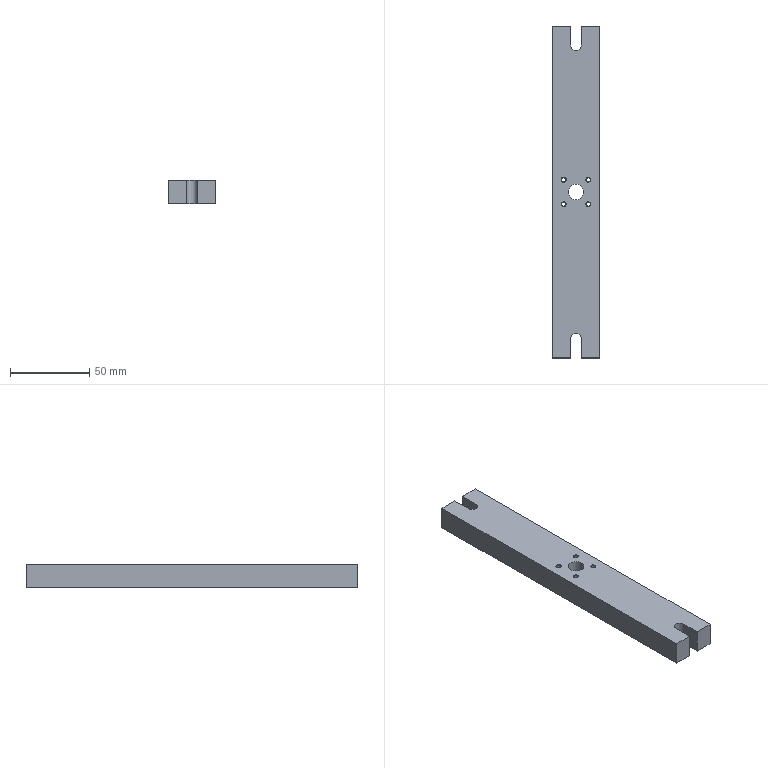Part | STEP file | 200 mesh_id1942 | 1 solid | 32 faces | box 30 x 210 x 15 mm | volume 89577 mm3 | plane 16 | cylinder 11 | cone 5 | commonest cylinder face diameters 2.5 x4 4.5 x4 7 x2 10 x1
STEP:
#1=CARTESIAN_POINT('',(-16645.224,-4012.519,101.75));
#2=VERTEX_POINT('',#1);
#3=CARTESIAN_POINT('',(-16643.974,-4012.519,101.75));
#4=DIRECTION('',(0.,0.,1.));
#5=DIRECTION('',(-1.,0.,0.));
#6=AXIS2_PLACEMENT_3D('',#3,#4,#5);
#7=CIRCLE('',#6,1.25);
#8=EDGE_CURVE('',#2,#2,#7,.T.);
#9=ORIENTED_EDGE('',*,*,#8,.T.);
#10=EDGE_LOOP('',(#9));
#11=FACE_BOUND('',#10,.T.);
#12=CARTESIAN_POINT('',(-16645.224,-4012.519,95.));
#13=VERTEX_POINT('',#12);
#14=CARTESIAN_POINT('',(-16643.974,-4012.519,95.));
#15=DIRECTION('',(0.,0.,1.));
#16=DIRECTION('',(-1.,0.,0.));
#17=AXIS2_PLACEMENT_3D('',#14,#15,#16);
#18=CIRCLE('',#17,1.25);
#19=EDGE_CURVE('',#13,#13,#18,.T.);
#20=ORIENTED_EDGE('',*,*,#19,.F.);
#21=EDGE_LOOP('',(#20));
#22=FACE_BOUND('',#21,.T.);
#23=CARTESIAN_POINT('',(-16643.974,-4012.519,102.));
#24=DIRECTION('',(0.,0.,-1.));
#25=DIRECTION('',(-1.,0.,0.));
#26=AXIS2_PLACEMENT_3D('',#23,#24,#25);
#27=CYLINDRICAL_SURFACE('',#26,1.25);
#28=ADVANCED_FACE('',(#11,#22),#27,.F.);
#29=CARTESIAN_POINT('',(-16629.724,-4012.519,101.75));
#30=VERTEX_POINT('',#29);
#31=CARTESIAN_POINT('',(-16628.474,-4012.519,101.75));
#32=DIRECTION('',(0.,0.,1.));
#33=DIRECTION('',(-1.,0.,0.));
#34=AXIS2_PLACEMENT_3D('',#31,#32,#33);
#35=CIRCLE('',#34,1.25);
#36=EDGE_CURVE('',#30,#30,#35,.T.);
#37=ORIENTED_EDGE('',*,*,#36,.T.);
#38=EDGE_LOOP('',(#37));
#39=FACE_BOUND('',#38,.T.);
#40=CARTESIAN_POINT('',(-16629.724,-4012.519,95.));
#41=VERTEX_POINT('',#40);
#42=CARTESIAN_POINT('',(-16628.474,-4012.519,95.));
#43=DIRECTION('',(0.,0.,1.));
#44=DIRECTION('',(-1.,0.,0.));
#45=AXIS2_PLACEMENT_3D('',#42,#43,#44);
#46=CIRCLE('',#45,1.25);
#47=EDGE_CURVE('',#41,#41,#46,.T.);
#48=ORIENTED_EDGE('',*,*,#47,.F.);
#49=EDGE_LOOP('',(#48));
#50=FACE_BOUND('',#49,.T.);
#51=CARTESIAN_POINT('',(-16628.474,-4012.519,102.));
#52=DIRECTION('',(0.,0.,-1.));
#53=DIRECTION('',(-1.,0.,0.));
#54=AXIS2_PLACEMENT_3D('',#51,#52,#53);
#55=CYLINDRICAL_SURFACE('',#54,1.25);
#56=ADVANCED_FACE('',(#39,#50),#55,.F.);
#57=CARTESIAN_POINT('',(-16645.224,-4028.019,101.75));
#58=VERTEX_POINT('',#57);
#59=CARTESIAN_POINT('',(-16643.974,-4028.019,101.75));
#60=DIRECTION('',(0.,0.,1.));
#61=DIRECTION('',(-1.,0.,0.));
#62=AXIS2_PLACEMENT_3D('',#59,#60,#61);
#63=CIRCLE('',#62,1.25);
#64=EDGE_CURVE('',#58,#58,#63,.T.);
#65=ORIENTED_EDGE('',*,*,#64,.T.);
#66=EDGE_LOOP('',(#65));
#67=FACE_BOUND('',#66,.T.);
#68=CARTESIAN_POINT('',(-16645.224,-4028.019,95.));
#69=VERTEX_POINT('',#68);
#70=CARTESIAN_POINT('',(-16643.974,-4028.019,95.));
#71=DIRECTION('',(0.,0.,1.));
#72=DIRECTION('',(-1.,0.,0.));
#73=AXIS2_PLACEMENT_3D('',#70,#71,#72);
#74=CIRCLE('',#73,1.25);
#75=EDGE_CURVE('',#69,#69,#74,.T.);
#76=ORIENTED_EDGE('',*,*,#75,.F.);
#77=EDGE_LOOP('',(#76));
#78=FACE_BOUND('',#77,.T.);
#79=CARTESIAN_POINT('',(-16643.974,-4028.019,102.));
#80=DIRECTION('',(0.,0.,-1.));
#81=DIRECTION('',(-1.,0.,0.));
#82=AXIS2_PLACEMENT_3D('',#79,#80,#81);
#83=CYLINDRICAL_SURFACE('',#82,1.25);
#84=ADVANCED_FACE('',(#67,#78),#83,.F.);
#85=CARTESIAN_POINT('',(-16629.724,-4028.019,101.75));
#86=VERTEX_POINT('',#85);
#87=CARTESIAN_POINT('',(-16628.474,-4028.019,101.75));
#88=DIRECTION('',(0.,0.,1.));
#89=DIRECTION('',(-1.,0.,0.));
#90=AXIS2_PLACEMENT_3D('',#87,#88,#89);
#91=CIRCLE('',#90,1.25);
#92=EDGE_CURVE('',#86,#86,#91,.T.);
#93=ORIENTED_EDGE('',*,*,#92,.T.);
#94=EDGE_LOOP('',(#93));
#95=FACE_BOUND('',#94,.T.);
#96=CARTESIAN_POINT('',(-16629.724,-4028.019,95.));
#97=VERTEX_POINT('',#96);
#98=CARTESIAN_POINT('',(-16628.474,-4028.019,95.));
#99=DIRECTION('',(0.,0.,1.));
#100=DIRECTION('',(-1.,0.,0.));
#101=AXIS2_PLACEMENT_3D('',#98,#99,#100);
#102=CIRCLE('',#101,1.25);
#103=EDGE_CURVE('',#97,#97,#102,.T.);
#104=ORIENTED_EDGE('',*,*,#103,.F.);
#105=EDGE_LOOP('',(#104));
#106=FACE_BOUND('',#105,.T.);
#107=CARTESIAN_POINT('',(-16628.474,-4028.019,102.));
#108=DIRECTION('',(0.,0.,-1.));
#109=DIRECTION('',(-1.,0.,0.));
#110=AXIS2_PLACEMENT_3D('',#107,#108,#109);
#111=CYLINDRICAL_SURFACE('',#110,1.25);
#112=ADVANCED_FACE('',(#95,#106),#111,.F.);
#113=CARTESIAN_POINT('',(-16639.724,-3927.269,102.));
#114=VERTEX_POINT('',#113);
#115=CARTESIAN_POINT('',(-16639.724,-3927.269,87.));
#116=VERTEX_POINT('',#115);
#117=CARTESIAN_POINT('',(-16639.724,-3927.269,146.));
#118=DIRECTION('',(0.,0.,-1.));
#119=VECTOR('',#118,1.);
#120=LINE('',#117,#119);
#121=EDGE_CURVE('',#114,#116,#120,.T.);
#122=ORIENTED_EDGE('',*,*,#121,.T.);
#123=CARTESIAN_POINT('',(-16639.724,-3915.269,87.));
#124=VERTEX_POINT('',#123);
#125=CARTESIAN_POINT('',(-16639.724,-3907.666,87.));
#126=DIRECTION('',(0.,-1.,0.));
#127=VECTOR('',#126,1.);
#128=LINE('',#125,#127);
#129=EDGE_CURVE('',#124,#116,#128,.T.);
#130=ORIENTED_EDGE('',*,*,#129,.F.);
#131=CARTESIAN_POINT('',(-16639.724,-3915.269,102.));
#132=VERTEX_POINT('',#131);
#133=CARTESIAN_POINT('',(-16639.724,-3915.269,146.));
#134=DIRECTION('',(0.,0.,-1.));
#135=VECTOR('',#134,1.);
#136=LINE('',#133,#135);
#137=EDGE_CURVE('',#132,#124,#136,.T.);
#138=ORIENTED_EDGE('',*,*,#137,.F.);
#139=CARTESIAN_POINT('',(-16639.724,-3907.666,102.));
#140=DIRECTION('',(0.,1.,0.));
#141=VECTOR('',#140,1.);
#142=LINE('',#139,#141);
#143=EDGE_CURVE('',#114,#132,#142,.T.);
#144=ORIENTED_EDGE('',*,*,#143,.F.);
#145=EDGE_LOOP('',(#122,#130,#138,#144));
#146=FACE_OUTER_BOUND('',#145,.T.);
#147=CARTESIAN_POINT('',(-16639.724,-3907.666,146.));
#148=DIRECTION('',(-1.,0.,0.));
#149=DIRECTION('',(0.,0.,1.));
#150=AXIS2_PLACEMENT_3D('',#147,#148,#149);
#151=PLANE('',#150);
#152=ADVANCED_FACE('',(#146),#151,.F.);
#153=CARTESIAN_POINT('',(-16632.724,-3915.269,87.));
#154=VERTEX_POINT('',#153);
#155=CARTESIAN_POINT('',(-16632.724,-3915.269,102.));
#156=VERTEX_POINT('',#155);
#157=CARTESIAN_POINT('',(-16632.724,-3915.269,146.));
#158=DIRECTION('',(0.,0.,1.));
#159=VECTOR('',#158,1.);
#160=LINE('',#157,#159);
#161=EDGE_CURVE('',#154,#156,#160,.T.);
#162=ORIENTED_EDGE('',*,*,#161,.F.);
#163=CARTESIAN_POINT('',(-16632.724,-3927.269,87.));
#164=VERTEX_POINT('',#163);
#165=CARTESIAN_POINT('',(-16632.724,-3927.269,87.));
#166=DIRECTION('',(0.,1.,0.));
#167=VECTOR('',#166,1.);
#168=LINE('',#165,#167);
#169=EDGE_CURVE('',#164,#154,#168,.T.);
#170=ORIENTED_EDGE('',*,*,#169,.F.);
#171=CARTESIAN_POINT('',(-16632.724,-3927.269,102.));
#172=VERTEX_POINT('',#171);
#173=CARTESIAN_POINT('',(-16632.724,-3927.269,146.));
#174=DIRECTION('',(0.,0.,-1.));
#175=VECTOR('',#174,1.);
#176=LINE('',#173,#175);
#177=EDGE_CURVE('',#172,#164,#176,.T.);
#178=ORIENTED_EDGE('',*,*,#177,.F.);
#179=CARTESIAN_POINT('',(-16632.724,-3927.269,102.));
#180=DIRECTION('',(0.,-1.,0.));
#181=VECTOR('',#180,1.);
#182=LINE('',#179,#181);
#183=EDGE_CURVE('',#156,#172,#182,.T.);
#184=ORIENTED_EDGE('',*,*,#183,.F.);
#185=EDGE_LOOP('',(#162,#170,#178,#184));
#186=FACE_OUTER_BOUND('',#185,.T.);
#187=CARTESIAN_POINT('',(-16632.724,-3927.269,146.));
#188=DIRECTION('',(1.,0.,0.));
#189=DIRECTION('',(0.,0.,-1.));
#190=AXIS2_PLACEMENT_3D('',#187,#188,#189);
#191=PLANE('',#190);
#192=ADVANCED_FACE('',(#186),#191,.F.);
#193=ORIENTED_EDGE('',*,*,#177,.T.);
#194=CARTESIAN_POINT('',(-16636.224,-3927.269,87.));
#195=DIRECTION('',(0.,0.,-1.));
#196=DIRECTION('',(-1.,0.,0.));
#197=AXIS2_PLACEMENT_3D('',#194,#195,#196);
#198=CIRCLE('',#197,3.5);
#199=EDGE_CURVE('',#164,#116,#198,.T.);
#200=ORIENTED_EDGE('',*,*,#199,.T.);
#201=ORIENTED_EDGE('',*,*,#121,.F.);
#202=CARTESIAN_POINT('',(-16636.224,-3927.269,102.));
#203=DIRECTION('',(0.,0.,-1.));
#204=DIRECTION('',(-1.,0.,0.));
#205=AXIS2_PLACEMENT_3D('',#202,#203,#204);
#206=CIRCLE('',#205,3.5);
#207=EDGE_CURVE('',#172,#114,#206,.T.);
#208=ORIENTED_EDGE('',*,*,#207,.F.);
#209=EDGE_LOOP('',(#193,#200,#201,#208));
#210=FACE_OUTER_BOUND('',#209,.T.);
#211=CARTESIAN_POINT('',(-16636.224,-3927.269,146.));
#212=DIRECTION('',(0.,0.,-1.));
#213=DIRECTION('',(-1.,0.,0.));
#214=AXIS2_PLACEMENT_3D('',#211,#212,#213);
#215=CYLINDRICAL_SURFACE('',#214,3.5);
#216=ADVANCED_FACE('',(#210),#215,.F.);
#217=CARTESIAN_POINT('',(-16642.615,-4012.519,101.859));
#218=VERTEX_POINT('',#217);
#219=CARTESIAN_POINT('',(-16643.974,-4012.519,101.859));
#220=DIRECTION('',(0.,0.,1.));
#221=DIRECTION('',(1.,0.,0.));
#222=AXIS2_PLACEMENT_3D('',#219,#220,#221);
#223=CIRCLE('',#222,1.359);
#224=EDGE_CURVE('',#218,#218,#223,.T.);
#225=ORIENTED_EDGE('',*,*,#224,.T.);
#226=EDGE_LOOP('',(#225));
#227=FACE_BOUND('',#226,.T.);
#228=ORIENTED_EDGE('',*,*,#8,.F.);
#229=EDGE_LOOP('',(#228));
#230=FACE_BOUND('',#229,.T.);
#231=CARTESIAN_POINT('',(-16643.974,-4012.519,102.));
#232=DIRECTION('',(0.,0.,1.));
#233=DIRECTION('',(1.,0.,0.));
#234=AXIS2_PLACEMENT_3D('',#231,#232,#233);
#235=CONICAL_SURFACE('',#234,1.5,45.);
#236=ADVANCED_FACE('',(#227,#230),#235,.F.);
#237=CARTESIAN_POINT('',(-16641.224,-4020.269,87.));
#238=VERTEX_POINT('',#237);
#239=CARTESIAN_POINT('',(-16636.224,-4020.269,87.));
#240=DIRECTION('',(0.,0.,-1.));
#241=DIRECTION('',(-1.,0.,0.));
#242=AXIS2_PLACEMENT_3D('',#239,#240,#241);
#243=CIRCLE('',#242,5.);
#244=EDGE_CURVE('',#238,#238,#243,.T.);
#245=ORIENTED_EDGE('',*,*,#244,.T.);
#246=EDGE_LOOP('',(#245));
#247=FACE_BOUND('',#246,.T.);
#248=CARTESIAN_POINT('',(-16641.224,-4020.269,102.));
#249=VERTEX_POINT('',#248);
#250=CARTESIAN_POINT('',(-16636.224,-4020.269,102.));
#251=DIRECTION('',(0.,0.,-1.));
#252=DIRECTION('',(-1.,0.,0.));
#253=AXIS2_PLACEMENT_3D('',#250,#251,#252);
#254=CIRCLE('',#253,5.);
#255=EDGE_CURVE('',#249,#249,#254,.T.);
#256=ORIENTED_EDGE('',*,*,#255,.F.);
#257=EDGE_LOOP('',(#256));
#258=FACE_BOUND('',#257,.T.);
#259=CARTESIAN_POINT('',(-16636.224,-4020.269,105.));
#260=DIRECTION('',(0.,0.,-1.));
#261=DIRECTION('',(1.,0.,0.));
#262=AXIS2_PLACEMENT_3D('',#259,#260,#261);
#263=CYLINDRICAL_SURFACE('',#262,5.);
#264=ADVANCED_FACE('',(#247,#258),#263,.F.);
#265=ORIENTED_EDGE('',*,*,#36,.F.);
#266=EDGE_LOOP('',(#265));
#267=FACE_BOUND('',#266,.T.);
#268=CARTESIAN_POINT('',(-16629.974,-4012.519,102.));
#269=VERTEX_POINT('',#268);
#270=CARTESIAN_POINT('',(-16628.474,-4012.519,102.));
#271=DIRECTION('',(0.,0.,-1.));
#272=DIRECTION('',(-1.,0.,0.));
#273=AXIS2_PLACEMENT_3D('',#270,#271,#272);
#274=CIRCLE('',#273,1.5);
#275=EDGE_CURVE('',#269,#269,#274,.T.);
#276=ORIENTED_EDGE('',*,*,#275,.F.);
#277=EDGE_LOOP('',(#276));
#278=FACE_BOUND('',#277,.T.);
#279=CARTESIAN_POINT('',(-16628.474,-4012.519,102.));
#280=DIRECTION('',(0.,0.,1.));
#281=DIRECTION('',(1.,0.,0.));
#282=AXIS2_PLACEMENT_3D('',#279,#280,#281);
#283=CONICAL_SURFACE('',#282,1.5,45.);
#284=ADVANCED_FACE('',(#267,#278),#283,.F.);
#285=ORIENTED_EDGE('',*,*,#64,.F.);
#286=EDGE_LOOP('',(#285));
#287=FACE_BOUND('',#286,.T.);
#288=CARTESIAN_POINT('',(-16645.474,-4028.019,102.));
#289=VERTEX_POINT('',#288);
#290=CARTESIAN_POINT('',(-16643.974,-4028.019,102.));
#291=DIRECTION('',(0.,0.,-1.));
#292=DIRECTION('',(-1.,0.,0.));
#293=AXIS2_PLACEMENT_3D('',#290,#291,#292);
#294=CIRCLE('',#293,1.5);
#295=EDGE_CURVE('',#289,#289,#294,.T.);
#296=ORIENTED_EDGE('',*,*,#295,.F.);
#297=EDGE_LOOP('',(#296));
#298=FACE_BOUND('',#297,.T.);
#299=CARTESIAN_POINT('',(-16643.974,-4028.019,102.));
#300=DIRECTION('',(0.,0.,1.));
#301=DIRECTION('',(1.,0.,0.));
#302=AXIS2_PLACEMENT_3D('',#299,#300,#301);
#303=CONICAL_SURFACE('',#302,1.5,45.);
#304=ADVANCED_FACE('',(#287,#298),#303,.F.);
#305=ORIENTED_EDGE('',*,*,#92,.F.);
#306=EDGE_LOOP('',(#305));
#307=FACE_BOUND('',#306,.T.);
#308=CARTESIAN_POINT('',(-16629.974,-4028.019,102.));
#309=VERTEX_POINT('',#308);
#310=CARTESIAN_POINT('',(-16628.474,-4028.019,102.));
#311=DIRECTION('',(0.,0.,-1.));
#312=DIRECTION('',(-1.,0.,0.));
#313=AXIS2_PLACEMENT_3D('',#310,#311,#312);
#314=CIRCLE('',#313,1.5);
#315=EDGE_CURVE('',#309,#309,#314,.T.);
#316=ORIENTED_EDGE('',*,*,#315,.F.);
#317=EDGE_LOOP('',(#316));
#318=FACE_BOUND('',#317,.T.);
#319=CARTESIAN_POINT('',(-16628.474,-4028.019,102.));
#320=DIRECTION('',(0.,0.,1.));
#321=DIRECTION('',(1.,0.,0.));
#322=AXIS2_PLACEMENT_3D('',#319,#320,#321);
#323=CONICAL_SURFACE('',#322,1.5,45.);
#324=ADVANCED_FACE('',(#307,#318),#323,.F.);
#325=ORIENTED_EDGE('',*,*,#224,.F.);
#326=EDGE_LOOP('',(#325));
#327=FACE_BOUND('',#326,.T.);
#328=CARTESIAN_POINT('',(-16645.674,-4012.519,102.));
#329=VERTEX_POINT('',#328);
#330=CARTESIAN_POINT('',(-16643.974,-4012.519,102.));
#331=DIRECTION('',(0.,0.,-1.));
#332=DIRECTION('',(-1.,0.,0.));
#333=AXIS2_PLACEMENT_3D('',#330,#331,#332);
#334=CIRCLE('',#333,1.7);
#335=EDGE_CURVE('',#329,#329,#334,.T.);
#336=ORIENTED_EDGE('',*,*,#335,.F.);
#337=EDGE_LOOP('',(#336));
#338=FACE_BOUND('',#337,.T.);
#339=CARTESIAN_POINT('',(-16643.974,-4012.519,102.));
#340=DIRECTION('',(0.,0.,1.));
#341=DIRECTION('',(1.,0.,0.));
#342=AXIS2_PLACEMENT_3D('',#339,#340,#341);
#343=CONICAL_SURFACE('',#342,1.7,67.5);
#344=ADVANCED_FACE('',(#327,#338),#343,.F.);
#345=CARTESIAN_POINT('',(-16621.224,-3915.269,87.));
#346=VERTEX_POINT('',#345);
#347=CARTESIAN_POINT('',(-16621.224,-4125.269,87.));
#348=VERTEX_POINT('',#347);
#349=CARTESIAN_POINT('',(-16621.224,-0.000000006,87.));
#350=DIRECTION('',(0.,-1.,0.));
#351=VECTOR('',#350,1.);
#352=LINE('',#349,#351);
#353=EDGE_CURVE('',#346,#348,#352,.T.);
#354=ORIENTED_EDGE('',*,*,#353,.F.);
#355=CARTESIAN_POINT('',(-16621.224,-3915.269,102.));
#356=VERTEX_POINT('',#355);
#357=CARTESIAN_POINT('',(-16621.224,-3915.269,105.));
#358=DIRECTION('',(0.,0.,-1.));
#359=VECTOR('',#358,1.);
#360=LINE('',#357,#359);
#361=EDGE_CURVE('',#356,#346,#360,.T.);
#362=ORIENTED_EDGE('',*,*,#361,.F.);
#363=CARTESIAN_POINT('',(-16621.224,-4125.269,102.));
#364=VERTEX_POINT('',#363);
#365=CARTESIAN_POINT('',(-16621.224,-0.000000006,102.));
#366=DIRECTION('',(0.,-1.,0.));
#367=VECTOR('',#366,1.);
#368=LINE('',#365,#367);
#369=EDGE_CURVE('',#356,#364,#368,.T.);
#370=ORIENTED_EDGE('',*,*,#369,.T.);
#371=CARTESIAN_POINT('',(-16621.224,-4125.269,105.));
#372=DIRECTION('',(0.,0.,-1.));
#373=VECTOR('',#372,1.);
#374=LINE('',#371,#373);
#375=EDGE_CURVE('',#364,#348,#374,.T.);
#376=ORIENTED_EDGE('',*,*,#375,.T.);
#377=EDGE_LOOP('',(#354,#362,#370,#376));
#378=FACE_OUTER_BOUND('',#377,.T.);
#379=CARTESIAN_POINT('',(-16621.224,-3915.269,105.));
#380=DIRECTION('',(1.,0.,0.));
#381=DIRECTION('',(0.,1.,0.));
#382=AXIS2_PLACEMENT_3D('',#379,#380,#381);
#383=PLANE('',#382);
#384=ADVANCED_FACE('',(#378),#383,.T.);
#385=CARTESIAN_POINT('',(-16632.724,-4125.269,102.));
#386=VERTEX_POINT('',#385);
#387=CARTESIAN_POINT('',(87.962,-4125.269,102.));
#388=DIRECTION('',(-1.,0.,0.));
#389=VECTOR('',#388,1.);
#390=LINE('',#387,#389);
#391=EDGE_CURVE('',#364,#386,#390,.T.);
#392=ORIENTED_EDGE('',*,*,#391,.T.);
#393=CARTESIAN_POINT('',(-16632.724,-4125.269,87.));
#394=VERTEX_POINT('',#393);
#395=CARTESIAN_POINT('',(-16632.724,-4125.269,146.));
#396=DIRECTION('',(0.,0.,-1.));
#397=VECTOR('',#396,1.);
#398=LINE('',#395,#397);
#399=EDGE_CURVE('',#386,#394,#398,.T.);
#400=ORIENTED_EDGE('',*,*,#399,.T.);
#401=CARTESIAN_POINT('',(87.962,-4125.269,87.));
#402=DIRECTION('',(-1.,0.,0.));
#403=VECTOR('',#402,1.);
#404=LINE('',#401,#403);
#405=EDGE_CURVE('',#348,#394,#404,.T.);
#406=ORIENTED_EDGE('',*,*,#405,.F.);
#407=ORIENTED_EDGE('',*,*,#375,.F.);
#408=EDGE_LOOP('',(#392,#400,#406,#407));
#409=FACE_OUTER_BOUND('',#408,.T.);
#410=CARTESIAN_POINT('',(-16621.224,-4125.269,105.));
#411=DIRECTION('',(0.,-1.,0.));
#412=DIRECTION('',(0.,0.,-1.));
#413=AXIS2_PLACEMENT_3D('',#410,#411,#412);
#414=PLANE('',#413);
#415=ADVANCED_FACE('',(#409),#414,.T.);
#416=ORIENTED_EDGE('',*,*,#399,.F.);
#417=CARTESIAN_POINT('',(-16632.724,-4113.269,102.));
#418=VERTEX_POINT('',#417);
#419=CARTESIAN_POINT('',(-16632.724,-4113.269,102.));
#420=DIRECTION('',(0.,-1.,0.));
#421=VECTOR('',#420,1.);
#422=LINE('',#419,#421);
#423=EDGE_CURVE('',#418,#386,#422,.T.);
#424=ORIENTED_EDGE('',*,*,#423,.F.);
#425=CARTESIAN_POINT('',(-16632.724,-4113.269,87.));
#426=VERTEX_POINT('',#425);
#427=CARTESIAN_POINT('',(-16632.724,-4113.269,146.));
#428=DIRECTION('',(0.,0.,1.));
#429=VECTOR('',#428,1.);
#430=LINE('',#427,#429);
#431=EDGE_CURVE('',#426,#418,#430,.T.);
#432=ORIENTED_EDGE('',*,*,#431,.F.);
#433=CARTESIAN_POINT('',(-16632.724,-4113.269,87.));
#434=DIRECTION('',(0.,1.,0.));
#435=VECTOR('',#434,1.);
#436=LINE('',#433,#435);
#437=EDGE_CURVE('',#394,#426,#436,.T.);
#438=ORIENTED_EDGE('',*,*,#437,.F.);
#439=EDGE_LOOP('',(#416,#424,#432,#438));
#440=FACE_OUTER_BOUND('',#439,.T.);
#441=CARTESIAN_POINT('',(-16632.724,-4113.269,146.));
#442=DIRECTION('',(1.,0.,0.));
#443=DIRECTION('',(0.,0.,-1.));
#444=AXIS2_PLACEMENT_3D('',#441,#442,#443);
#445=PLANE('',#444);
#446=ADVANCED_FACE('',(#440),#445,.F.);
#447=ORIENTED_EDGE('',*,*,#431,.T.);
#448=CARTESIAN_POINT('',(-16639.724,-4113.269,102.));
#449=VERTEX_POINT('',#448);
#450=CARTESIAN_POINT('',(-16636.224,-4113.269,102.));
#451=DIRECTION('',(0.,0.,-1.));
#452=DIRECTION('',(-1.,0.,0.));
#453=AXIS2_PLACEMENT_3D('',#450,#451,#452);
#454=CIRCLE('',#453,3.5);
#455=EDGE_CURVE('',#449,#418,#454,.T.);
#456=ORIENTED_EDGE('',*,*,#455,.F.);
#457=CARTESIAN_POINT('',(-16639.724,-4113.269,87.));
#458=VERTEX_POINT('',#457);
#459=CARTESIAN_POINT('',(-16639.724,-4113.269,146.));
#460=DIRECTION('',(0.,0.,1.));
#461=VECTOR('',#460,1.);
#462=LINE('',#459,#461);
#463=EDGE_CURVE('',#458,#449,#462,.T.);
#464=ORIENTED_EDGE('',*,*,#463,.F.);
#465=CARTESIAN_POINT('',(-16636.224,-4113.269,87.));
#466=DIRECTION('',(0.,0.,1.));
#467=DIRECTION('',(-1.,0.,0.));
#468=AXIS2_PLACEMENT_3D('',#465,#466,#467);
#469=CIRCLE('',#468,3.5);
#470=EDGE_CURVE('',#426,#458,#469,.T.);
#471=ORIENTED_EDGE('',*,*,#470,.F.);
#472=EDGE_LOOP('',(#447,#456,#464,#471));
#473=FACE_OUTER_BOUND('',#472,.T.);
#474=CARTESIAN_POINT('',(-16636.224,-4113.269,146.));
#475=DIRECTION('',(0.,0.,-1.));
#476=DIRECTION('',(-1.,0.,0.));
#477=AXIS2_PLACEMENT_3D('',#474,#475,#476);
#478=CYLINDRICAL_SURFACE('',#477,3.5);
#479=ADVANCED_FACE('',(#473),#478,.F.);
#480=ORIENTED_EDGE('',*,*,#463,.T.);
#481=CARTESIAN_POINT('',(-16639.724,-4125.269,102.));
#482=VERTEX_POINT('',#481);
#483=CARTESIAN_POINT('',(-16639.724,-4132.872,102.));
#484=DIRECTION('',(0.,1.,0.));
#485=VECTOR('',#484,1.);
#486=LINE('',#483,#485);
#487=EDGE_CURVE('',#482,#449,#486,.T.);
#488=ORIENTED_EDGE('',*,*,#487,.F.);
#489=CARTESIAN_POINT('',(-16639.724,-4125.269,87.));
#490=VERTEX_POINT('',#489);
#491=CARTESIAN_POINT('',(-16639.724,-4125.269,146.));
#492=DIRECTION('',(0.,0.,1.));
#493=VECTOR('',#492,1.);
#494=LINE('',#491,#493);
#495=EDGE_CURVE('',#490,#482,#494,.T.);
#496=ORIENTED_EDGE('',*,*,#495,.F.);
#497=CARTESIAN_POINT('',(-16639.724,-4132.872,87.));
#498=DIRECTION('',(0.,-1.,0.));
#499=VECTOR('',#498,1.);
#500=LINE('',#497,#499);
#501=EDGE_CURVE('',#458,#490,#500,.T.);
#502=ORIENTED_EDGE('',*,*,#501,.F.);
#503=EDGE_LOOP('',(#480,#488,#496,#502));
#504=FACE_OUTER_BOUND('',#503,.T.);
#505=CARTESIAN_POINT('',(-16639.724,-4132.872,146.));
#506=DIRECTION('',(-1.,0.,0.));
#507=DIRECTION('',(0.,0.,1.));
#508=AXIS2_PLACEMENT_3D('',#505,#506,#507);
#509=PLANE('',#508);
#510=ADVANCED_FACE('',(#504),#509,.F.);
#511=CARTESIAN_POINT('',(-16651.224,-4125.269,87.));
#512=VERTEX_POINT('',#511);
#513=CARTESIAN_POINT('',(87.962,-4125.269,87.));
#514=DIRECTION('',(-1.,0.,0.));
#515=VECTOR('',#514,1.);
#516=LINE('',#513,#515);
#517=EDGE_CURVE('',#490,#512,#516,.T.);
#518=ORIENTED_EDGE('',*,*,#517,.F.);
#519=ORIENTED_EDGE('',*,*,#495,.T.);
#520=CARTESIAN_POINT('',(-16651.224,-4125.269,102.));
#521=VERTEX_POINT('',#520);
#522=CARTESIAN_POINT('',(87.962,-4125.269,102.));
#523=DIRECTION('',(-1.,0.,0.));
#524=VECTOR('',#523,1.);
#525=LINE('',#522,#524);
#526=EDGE_CURVE('',#482,#521,#525,.T.);
#527=ORIENTED_EDGE('',*,*,#526,.T.);
#528=CARTESIAN_POINT('',(-16651.224,-4125.269,105.));
#529=DIRECTION('',(0.,0.,-1.));
#530=VECTOR('',#529,1.);
#531=LINE('',#528,#530);
#532=EDGE_CURVE('',#521,#512,#531,.T.);
#533=ORIENTED_EDGE('',*,*,#532,.T.);
#534=EDGE_LOOP('',(#518,#519,#527,#533));
#535=FACE_OUTER_BOUND('',#534,.T.);
#536=CARTESIAN_POINT('',(-16621.224,-4125.269,105.));
#537=DIRECTION('',(0.,-1.,0.));
#538=DIRECTION('',(0.,0.,-1.));
#539=AXIS2_PLACEMENT_3D('',#536,#537,#538);
#540=PLANE('',#539);
#541=ADVANCED_FACE('',(#535),#540,.T.);
#542=CARTESIAN_POINT('',(-16651.224,-3915.269,87.));
#543=VERTEX_POINT('',#542);
#544=CARTESIAN_POINT('',(-16651.224,0.000000002,87.));
#545=DIRECTION('',(0.,1.,0.));
#546=VECTOR('',#545,1.);
#547=LINE('',#544,#546);
#548=EDGE_CURVE('',#512,#543,#547,.T.);
#549=ORIENTED_EDGE('',*,*,#548,.F.);
#550=ORIENTED_EDGE('',*,*,#532,.F.);
#551=CARTESIAN_POINT('',(-16651.224,-3915.269,102.));
#552=VERTEX_POINT('',#551);
#553=CARTESIAN_POINT('',(-16651.224,0.000000002,102.));
#554=DIRECTION('',(0.,1.,0.));
#555=VECTOR('',#554,1.);
#556=LINE('',#553,#555);
#557=EDGE_CURVE('',#521,#552,#556,.T.);
#558=ORIENTED_EDGE('',*,*,#557,.T.);
#559=CARTESIAN_POINT('',(-16651.224,-3915.269,105.));
#560=DIRECTION('',(0.,0.,-1.));
#561=VECTOR('',#560,1.);
#562=LINE('',#559,#561);
#563=EDGE_CURVE('',#552,#543,#562,.T.);
#564=ORIENTED_EDGE('',*,*,#563,.T.);
#565=EDGE_LOOP('',(#549,#550,#558,#564));
#566=FACE_OUTER_BOUND('',#565,.T.);
#567=CARTESIAN_POINT('',(-16651.224,-4125.269,105.));
#568=DIRECTION('',(-1.,0.,0.));
#569=DIRECTION('',(0.,-1.,0.));
#570=AXIS2_PLACEMENT_3D('',#567,#568,#569);
#571=PLANE('',#570);
#572=ADVANCED_FACE('',(#566),#571,.T.);
#573=CARTESIAN_POINT('',(87.962,-3915.269,102.));
#574=DIRECTION('',(1.,0.,0.));
#575=VECTOR('',#574,1.);
#576=LINE('',#573,#575);
#577=EDGE_CURVE('',#552,#132,#576,.T.);
#578=ORIENTED_EDGE('',*,*,#577,.T.);
#579=ORIENTED_EDGE('',*,*,#137,.T.);
#580=CARTESIAN_POINT('',(87.962,-3915.269,87.));
#581=DIRECTION('',(1.,0.,0.));
#582=VECTOR('',#581,1.);
#583=LINE('',#580,#582);
#584=EDGE_CURVE('',#543,#124,#583,.T.);
#585=ORIENTED_EDGE('',*,*,#584,.F.);
#586=ORIENTED_EDGE('',*,*,#563,.F.);
#587=EDGE_LOOP('',(#578,#579,#585,#586));
#588=FACE_OUTER_BOUND('',#587,.T.);
#589=CARTESIAN_POINT('',(-16651.224,-3915.269,105.));
#590=DIRECTION('',(0.,1.,0.));
#591=DIRECTION('',(0.,0.,1.));
#592=AXIS2_PLACEMENT_3D('',#589,#590,#591);
#593=PLANE('',#592);
#594=ADVANCED_FACE('',(#588),#593,.T.);
#595=CARTESIAN_POINT('',(87.962,-3915.269,87.));
#596=DIRECTION('',(1.,0.,0.));
#597=VECTOR('',#596,1.);
#598=LINE('',#595,#597);
#599=EDGE_CURVE('',#154,#346,#598,.T.);
#600=ORIENTED_EDGE('',*,*,#599,.F.);
#601=ORIENTED_EDGE('',*,*,#161,.T.);
#602=CARTESIAN_POINT('',(87.962,-3915.269,102.));
#603=DIRECTION('',(1.,0.,0.));
#604=VECTOR('',#603,1.);
#605=LINE('',#602,#604);
#606=EDGE_CURVE('',#156,#356,#605,.T.);
#607=ORIENTED_EDGE('',*,*,#606,.T.);
#608=ORIENTED_EDGE('',*,*,#361,.T.);
#609=EDGE_LOOP('',(#600,#601,#607,#608));
#610=FACE_OUTER_BOUND('',#609,.T.);
#611=CARTESIAN_POINT('',(-16651.224,-3915.269,105.));
#612=DIRECTION('',(0.,1.,0.));
#613=DIRECTION('',(0.,0.,1.));
#614=AXIS2_PLACEMENT_3D('',#611,#612,#613);
#615=PLANE('',#614);
#616=ADVANCED_FACE('',(#610),#615,.T.);
#617=ORIENTED_EDGE('',*,*,#606,.F.);
#618=ORIENTED_EDGE('',*,*,#183,.T.);
#619=ORIENTED_EDGE('',*,*,#207,.T.);
#620=ORIENTED_EDGE('',*,*,#143,.T.);
#621=ORIENTED_EDGE('',*,*,#577,.F.);
#622=ORIENTED_EDGE('',*,*,#557,.F.);
#623=ORIENTED_EDGE('',*,*,#526,.F.);
#624=ORIENTED_EDGE('',*,*,#487,.T.);
#625=ORIENTED_EDGE('',*,*,#455,.T.);
#626=ORIENTED_EDGE('',*,*,#423,.T.);
#627=ORIENTED_EDGE('',*,*,#391,.F.);
#628=ORIENTED_EDGE('',*,*,#369,.F.);
#629=EDGE_LOOP('',(#617,#618,#619,#620,#621,#622,#623,#624,#625,#626,#627,#628));
#630=FACE_BOUND('',#629,.T.);
#631=ORIENTED_EDGE('',*,*,#335,.T.);
#632=EDGE_LOOP('',(#631));
#633=FACE_BOUND('',#632,.T.);
#634=ORIENTED_EDGE('',*,*,#315,.T.);
#635=EDGE_LOOP('',(#634));
#636=FACE_BOUND('',#635,.T.);
#637=ORIENTED_EDGE('',*,*,#295,.T.);
#638=EDGE_LOOP('',(#637));
#639=FACE_BOUND('',#638,.T.);
#640=ORIENTED_EDGE('',*,*,#275,.T.);
#641=EDGE_LOOP('',(#640));
#642=FACE_BOUND('',#641,.T.);
#643=ORIENTED_EDGE('',*,*,#255,.T.);
#644=EDGE_LOOP('',(#643));
#645=FACE_BOUND('',#644,.T.);
#646=CARTESIAN_POINT('',(87.962,0.,102.));
#647=DIRECTION('',(0.,0.,-1.));
#648=DIRECTION('',(-1.,0.,0.));
#649=AXIS2_PLACEMENT_3D('',#646,#647,#648);
#650=PLANE('',#649);
#651=ADVANCED_FACE('',(#630,#633,#636,#639,#642,#645),#650,.F.);
#652=CARTESIAN_POINT('',(-16630.724,-4012.519,87.));
#653=VERTEX_POINT('',#652);
#654=CARTESIAN_POINT('',(-16628.474,-4012.519,87.));
#655=DIRECTION('',(0.,0.,-1.));
#656=DIRECTION('',(-1.,0.,0.));
#657=AXIS2_PLACEMENT_3D('',#654,#655,#656);
#658=CIRCLE('',#657,2.25);
#659=EDGE_CURVE('',#653,#653,#658,.T.);
#660=ORIENTED_EDGE('',*,*,#659,.F.);
#661=EDGE_LOOP('',(#660));
#662=FACE_BOUND('',#661,.T.);
#663=CARTESIAN_POINT('',(-16646.224,-4012.519,87.));
#664=VERTEX_POINT('',#663);
#665=CARTESIAN_POINT('',(-16643.974,-4012.519,87.));
#666=DIRECTION('',(0.,0.,-1.));
#667=DIRECTION('',(-1.,0.,0.));
#668=AXIS2_PLACEMENT_3D('',#665,#666,#667);
#669=CIRCLE('',#668,2.25);
#670=EDGE_CURVE('',#664,#664,#669,.T.);
#671=ORIENTED_EDGE('',*,*,#670,.F.);
#672=EDGE_LOOP('',(#671));
#673=FACE_BOUND('',#672,.T.);
#674=CARTESIAN_POINT('',(-16646.224,-4028.019,87.));
#675=VERTEX_POINT('',#674);
#676=CARTESIAN_POINT('',(-16643.974,-4028.019,87.));
#677=DIRECTION('',(0.,0.,-1.));
#678=DIRECTION('',(-1.,0.,0.));
#679=AXIS2_PLACEMENT_3D('',#676,#677,#678);
#680=CIRCLE('',#679,2.25);
#681=EDGE_CURVE('',#675,#675,#680,.T.);
#682=ORIENTED_EDGE('',*,*,#681,.F.);
#683=EDGE_LOOP('',(#682));
#684=FACE_BOUND('',#683,.T.);
#685=CARTESIAN_POINT('',(-16630.724,-4028.019,87.));
#686=VERTEX_POINT('',#685);
#687=CARTESIAN_POINT('',(-16628.474,-4028.019,87.));
#688=DIRECTION('',(0.,0.,-1.));
#689=DIRECTION('',(-1.,0.,0.));
#690=AXIS2_PLACEMENT_3D('',#687,#688,#689);
#691=CIRCLE('',#690,2.25);
#692=EDGE_CURVE('',#686,#686,#691,.T.);
#693=ORIENTED_EDGE('',*,*,#692,.F.);
#694=EDGE_LOOP('',(#693));
#695=FACE_BOUND('',#694,.T.);
#696=ORIENTED_EDGE('',*,*,#244,.F.);
#697=EDGE_LOOP('',(#696));
#698=FACE_BOUND('',#697,.T.);
#699=ORIENTED_EDGE('',*,*,#199,.F.);
#700=ORIENTED_EDGE('',*,*,#169,.T.);
#701=ORIENTED_EDGE('',*,*,#599,.T.);
#702=ORIENTED_EDGE('',*,*,#353,.T.);
#703=ORIENTED_EDGE('',*,*,#405,.T.);
#704=ORIENTED_EDGE('',*,*,#437,.T.);
#705=ORIENTED_EDGE('',*,*,#470,.T.);
#706=ORIENTED_EDGE('',*,*,#501,.T.);
#707=ORIENTED_EDGE('',*,*,#517,.T.);
#708=ORIENTED_EDGE('',*,*,#548,.T.);
#709=ORIENTED_EDGE('',*,*,#584,.T.);
#710=ORIENTED_EDGE('',*,*,#129,.T.);
#711=EDGE_LOOP('',(#699,#700,#701,#702,#703,#704,#705,#706,#707,#708,#709,#710));
#712=FACE_BOUND('',#711,.T.);
#713=CARTESIAN_POINT('',(87.962,0.,87.));
#714=DIRECTION('',(0.,0.,-1.));
#715=DIRECTION('',(-1.,0.,0.));
#716=AXIS2_PLACEMENT_3D('',#713,#714,#715);
#717=PLANE('',#716);
#718=ADVANCED_FACE('',(#662,#673,#684,#695,#698,#712),#717,.T.);
#719=CARTESIAN_POINT('',(-16630.724,-4028.019,95.));
#720=VERTEX_POINT('',#719);
#721=CARTESIAN_POINT('',(-16628.474,-4028.019,95.));
#722=DIRECTION('',(0.,0.,1.));
#723=DIRECTION('',(-1.,0.,0.));
#724=AXIS2_PLACEMENT_3D('',#721,#722,#723);
#725=CIRCLE('',#724,2.25);
#726=EDGE_CURVE('',#720,#720,#725,.T.);
#727=ORIENTED_EDGE('',*,*,#726,.F.);
#728=EDGE_LOOP('',(#727));
#729=FACE_BOUND('',#728,.T.);
#730=ORIENTED_EDGE('',*,*,#103,.T.);
#731=EDGE_LOOP('',(#730));
#732=FACE_BOUND('',#731,.T.);
#733=CARTESIAN_POINT('',(-16628.474,-4028.019,95.));
#734=DIRECTION('',(0.,0.,-1.));
#735=DIRECTION('',(-1.,0.,0.));
#736=AXIS2_PLACEMENT_3D('',#733,#734,#735);
#737=PLANE('',#736);
#738=ADVANCED_FACE('',(#729,#732),#737,.T.);
#739=ORIENTED_EDGE('',*,*,#692,.T.);
#740=EDGE_LOOP('',(#739));
#741=FACE_BOUND('',#740,.T.);
#742=ORIENTED_EDGE('',*,*,#726,.T.);
#743=EDGE_LOOP('',(#742));
#744=FACE_BOUND('',#743,.T.);
#745=CARTESIAN_POINT('',(-16628.474,-4028.019,87.));
#746=DIRECTION('',(0.,0.,1.));
#747=DIRECTION('',(1.,0.,0.));
#748=AXIS2_PLACEMENT_3D('',#745,#746,#747);
#749=CYLINDRICAL_SURFACE('',#748,2.25);
#750=ADVANCED_FACE('',(#741,#744),#749,.F.);
#751=CARTESIAN_POINT('',(-16646.224,-4028.019,95.));
#752=VERTEX_POINT('',#751);
#753=CARTESIAN_POINT('',(-16643.974,-4028.019,95.));
#754=DIRECTION('',(0.,0.,1.));
#755=DIRECTION('',(-1.,0.,0.));
#756=AXIS2_PLACEMENT_3D('',#753,#754,#755);
#757=CIRCLE('',#756,2.25);
#758=EDGE_CURVE('',#752,#752,#757,.T.);
#759=ORIENTED_EDGE('',*,*,#758,.F.);
#760=EDGE_LOOP('',(#759));
#761=FACE_BOUND('',#760,.T.);
#762=ORIENTED_EDGE('',*,*,#75,.T.);
#763=EDGE_LOOP('',(#762));
#764=FACE_BOUND('',#763,.T.);
#765=CARTESIAN_POINT('',(-16643.974,-4028.019,95.));
#766=DIRECTION('',(0.,0.,-1.));
#767=DIRECTION('',(-1.,0.,0.));
#768=AXIS2_PLACEMENT_3D('',#765,#766,#767);
#769=PLANE('',#768);
#770=ADVANCED_FACE('',(#761,#764),#769,.T.);
#771=ORIENTED_EDGE('',*,*,#681,.T.);
#772=EDGE_LOOP('',(#771));
#773=FACE_BOUND('',#772,.T.);
#774=ORIENTED_EDGE('',*,*,#758,.T.);
#775=EDGE_LOOP('',(#774));
#776=FACE_BOUND('',#775,.T.);
#777=CARTESIAN_POINT('',(-16643.974,-4028.019,87.));
#778=DIRECTION('',(0.,0.,1.));
#779=DIRECTION('',(1.,0.,0.));
#780=AXIS2_PLACEMENT_3D('',#777,#778,#779);
#781=CYLINDRICAL_SURFACE('',#780,2.25);
#782=ADVANCED_FACE('',(#773,#776),#781,.F.);
#783=CARTESIAN_POINT('',(-16630.724,-4012.519,95.));
#784=VERTEX_POINT('',#783);
#785=CARTESIAN_POINT('',(-16628.474,-4012.519,95.));
#786=DIRECTION('',(0.,0.,1.));
#787=DIRECTION('',(-1.,0.,0.));
#788=AXIS2_PLACEMENT_3D('',#785,#786,#787);
#789=CIRCLE('',#788,2.25);
#790=EDGE_CURVE('',#784,#784,#789,.T.);
#791=ORIENTED_EDGE('',*,*,#790,.F.);
#792=EDGE_LOOP('',(#791));
#793=FACE_BOUND('',#792,.T.);
#794=ORIENTED_EDGE('',*,*,#47,.T.);
#795=EDGE_LOOP('',(#794));
#796=FACE_BOUND('',#795,.T.);
#797=CARTESIAN_POINT('',(-16628.474,-4012.519,95.));
#798=DIRECTION('',(0.,0.,-1.));
#799=DIRECTION('',(-1.,0.,0.));
#800=AXIS2_PLACEMENT_3D('',#797,#798,#799);
#801=PLANE('',#800);
#802=ADVANCED_FACE('',(#793,#796),#801,.T.);
#803=ORIENTED_EDGE('',*,*,#659,.T.);
#804=EDGE_LOOP('',(#803));
#805=FACE_BOUND('',#804,.T.);
#806=ORIENTED_EDGE('',*,*,#790,.T.);
#807=EDGE_LOOP('',(#806));
#808=FACE_BOUND('',#807,.T.);
#809=CARTESIAN_POINT('',(-16628.474,-4012.519,87.));
#810=DIRECTION('',(0.,0.,1.));
#811=DIRECTION('',(1.,0.,0.));
#812=AXIS2_PLACEMENT_3D('',#809,#810,#811);
#813=CYLINDRICAL_SURFACE('',#812,2.25);
#814=ADVANCED_FACE('',(#805,#808),#813,.F.);
#815=CARTESIAN_POINT('',(-16646.224,-4012.519,95.));
#816=VERTEX_POINT('',#815);
#817=CARTESIAN_POINT('',(-16643.974,-4012.519,95.));
#818=DIRECTION('',(0.,0.,1.));
#819=DIRECTION('',(-1.,0.,0.));
#820=AXIS2_PLACEMENT_3D('',#817,#818,#819);
#821=CIRCLE('',#820,2.25);
#822=EDGE_CURVE('',#816,#816,#821,.T.);
#823=ORIENTED_EDGE('',*,*,#822,.F.);
#824=EDGE_LOOP('',(#823));
#825=FACE_BOUND('',#824,.T.);
#826=ORIENTED_EDGE('',*,*,#19,.T.);
#827=EDGE_LOOP('',(#826));
#828=FACE_BOUND('',#827,.T.);
#829=CARTESIAN_POINT('',(-16643.974,-4012.519,95.));
#830=DIRECTION('',(0.,0.,-1.));
#831=DIRECTION('',(-1.,0.,0.));
#832=AXIS2_PLACEMENT_3D('',#829,#830,#831);
#833=PLANE('',#832);
#834=ADVANCED_FACE('',(#825,#828),#833,.T.);
#835=ORIENTED_EDGE('',*,*,#670,.T.);
#836=EDGE_LOOP('',(#835));
#837=FACE_BOUND('',#836,.T.);
#838=ORIENTED_EDGE('',*,*,#822,.T.);
#839=EDGE_LOOP('',(#838));
#840=FACE_BOUND('',#839,.T.);
#841=CARTESIAN_POINT('',(-16643.974,-4012.519,87.));
#842=DIRECTION('',(0.,0.,1.));
#843=DIRECTION('',(1.,0.,0.));
#844=AXIS2_PLACEMENT_3D('',#841,#842,#843);
#845=CYLINDRICAL_SURFACE('',#844,2.25);
#846=ADVANCED_FACE('',(#837,#840),#845,.F.);
#847=CLOSED_SHELL('',(#28,#56,#84,#112,#152,#192,#216,#236,#264,#284,#304,#324,#344,#384,#415,#446,#479,#510,#541,#572,#594,#616,#651,#718,#738,#750,#770,#782,#802,#814,#834,#846));
#848=MANIFOLD_SOLID_BREP('',#847);
#849=(LENGTH_UNIT()NAMED_UNIT(*)SI_UNIT(.MILLI.,.METRE.));
#850=UNCERTAINTY_MEASURE_WITH_UNIT(LENGTH_MEASURE(0.00002),#849,'','');
#851=(NAMED_UNIT(*)PLANE_ANGLE_UNIT()SI_UNIT($,.RADIAN.));
#852=PLANE_ANGLE_MEASURE_WITH_UNIT(PLANE_ANGLE_MEASURE(0.01745),#851);
#853=DIMENSIONAL_EXPONENTS(0.,0.,0.,0.,0.,0.,0.);
#854=(CONVERSION_BASED_UNIT('DEGREE',#852)NAMED_UNIT(#853)PLANE_ANGLE_UNIT());
#855=(NAMED_UNIT(*)SI_UNIT($,.STERADIAN.)SOLID_ANGLE_UNIT());
#856=(GEOMETRIC_REPRESENTATION_CONTEXT(3)GLOBAL_UNCERTAINTY_ASSIGNED_CONTEXT((#850))GLOBAL_UNIT_ASSIGNED_CONTEXT((#849,#854,#855))REPRESENTATION_CONTEXT('',''));
#857=ADVANCED_BREP_SHAPE_REPRESENTATION('',(#848),#856);